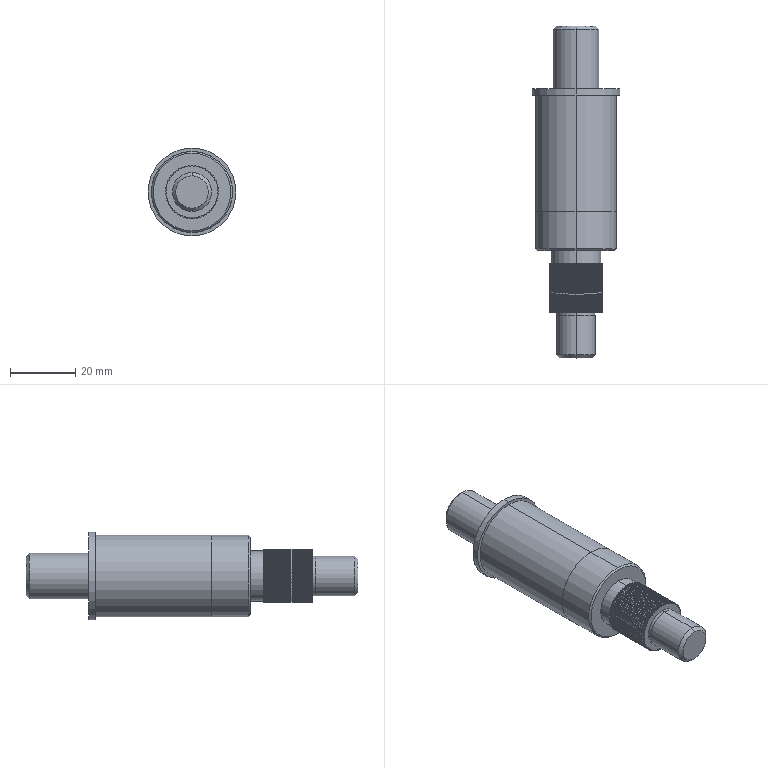Part | SolidWorks | features BaseBody 2 | 2 solids | 287 faces | box 27 x 101.9 x 27 mm | volume 32783 mm3 | cylinder 173 | plane 108 | cone 6 | commonest cylinder face diameters 0.75 x110 16.285 x49 12 x4 14 x2 15.4 x2 24.9 x2